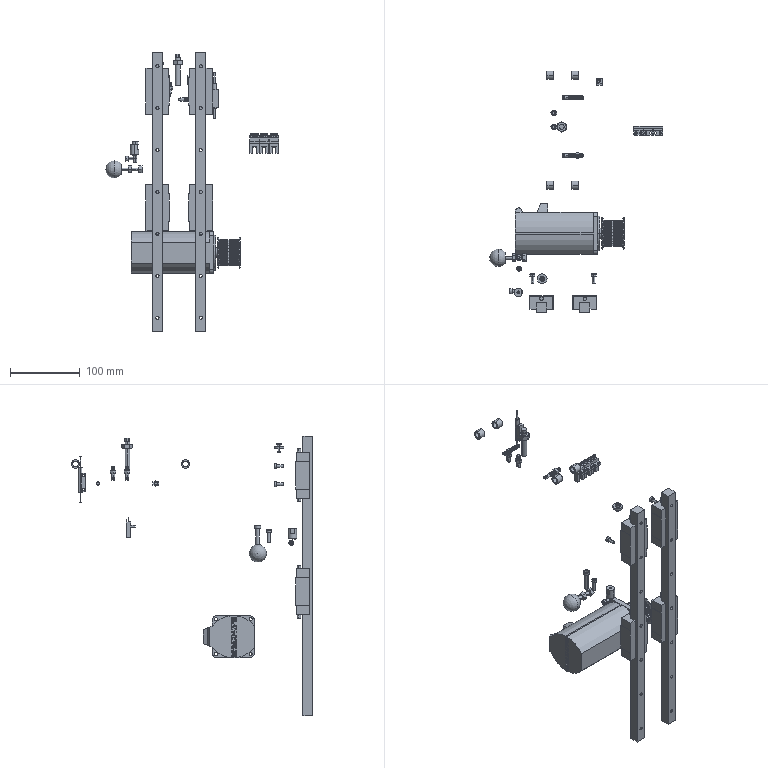Part | NX | 38 solids | 2503 faces | box 247.9 x 345.7 x 400 mm | volume 732314 mm3 | plane 1626 | cylinder 701 | cone 124 | spline 44 | sphere 8 | commonest cylinder face diameters 5 x193 0.5 x52 6.55 x52 1.1 x48 37.24 x48 4.5 x36